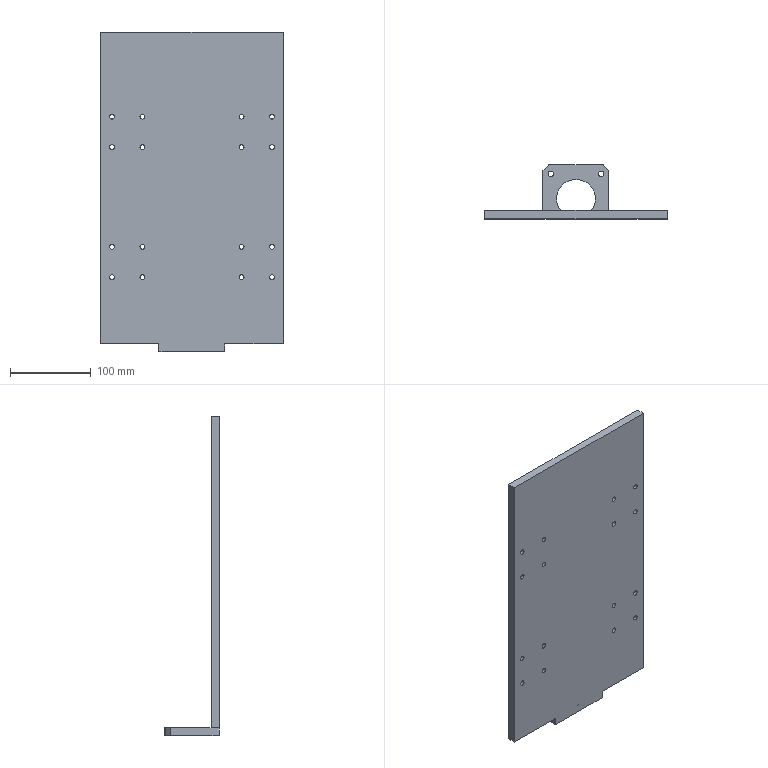Part | STEP file | 1 solid | 55 faces | box 225.075 x 66.921 x 394.223 mm | volume 895884 mm3 | cylinder 40 | plane 15 | commonest cylinder face diameters 6 x32 6.8 x4 2 x2 48 x2